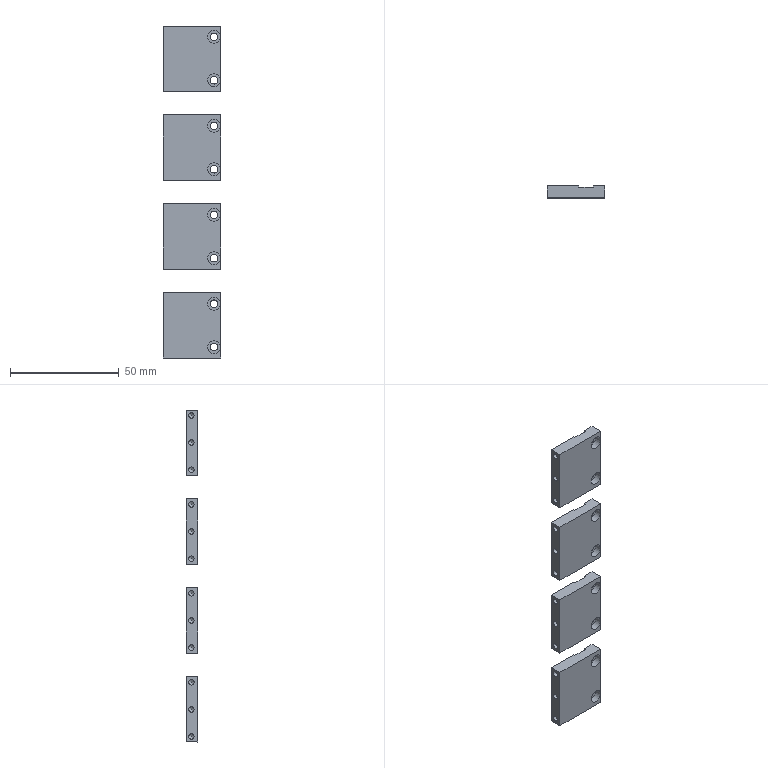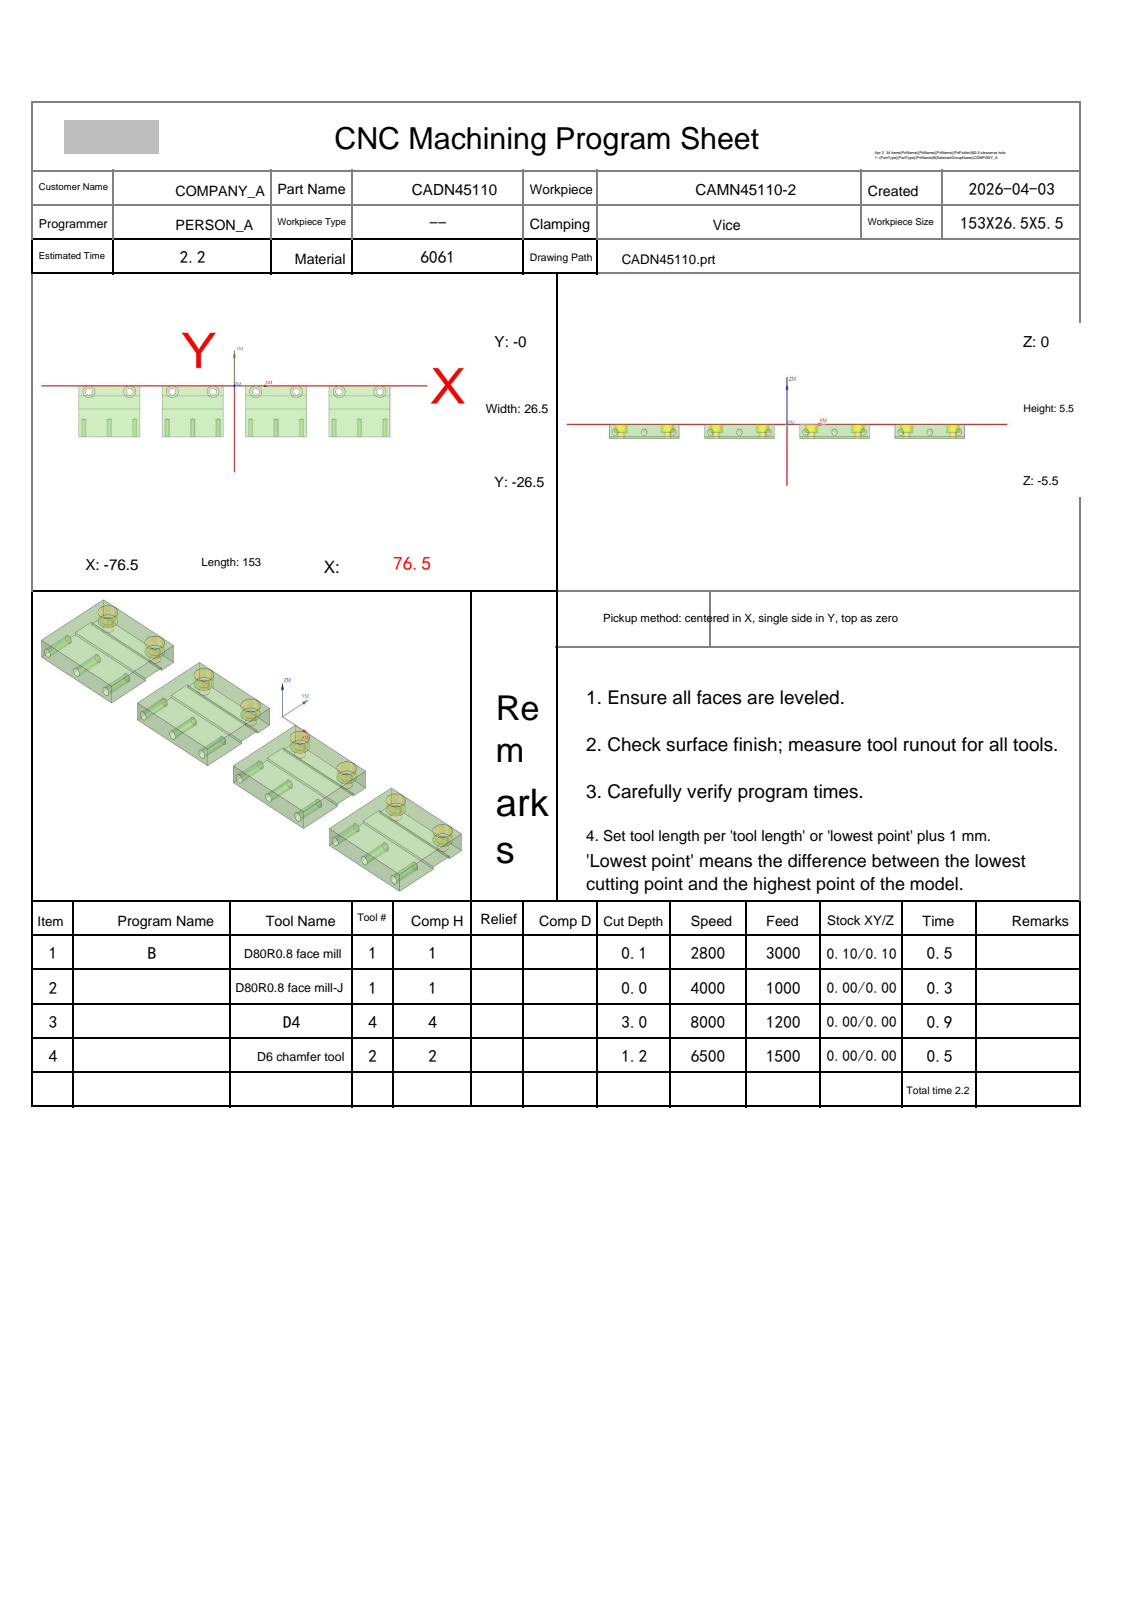NC program | NX | posted by the shop | part box 26.5 x 5.5 x 153 mm
Whole program:
%
O0001
(Machine time: 2.96 MIN)
(===Total Tool:3===)
(T1=D80R0.8 face mill D=80.  R=0.8  D-  H01 Z=-0.   )
(T4=D4      D=4.   R=0.   D-  H04 Z=-3.   )
(T2=D6 chamfer tool   D=6.   R=0.   D-  H02 Z=-1.2  )
G80 G90 G17 G49 G40
G91 G28 Z0
M01
N1 T01 M06
(D80R0.8 face mill  D=80. R=0.8 H=01 ce=0.10 di=0.10)
G00 G90 G54 X128.597 Y-13.25 M03 S2800
G43 H01 Z20.
M08
Z4.02
G01 Z2.02 F3000.
X116.597
X-116.597
X-128.597
Z4.02
G00 X128.597
Z3.54
G01 Z1.54
X116.597
X-116.597
X-128.597
Z3.54
G00 X128.597
Z3.06
G01 Z1.06
X116.597
X-116.597
X-128.597
Z3.06
G00 X128.597
Z2.58
G01 Z.58
X116.597
X-116.597
X-128.597
Z2.58
G00 Z20.
X128.597
Z2.1
G01 Z.1
X116.597
X-116.597
X-128.597
Z2.1
G00 Z20.
G91 G28 Z0.0
M05
M09
G91 G28 Z0.0
M01
N2 T01 M06
(D80R0.8 face mill-J  D=80. R=0.8 H=01 ce=0.00 di=0.00)
G00 G90 G54 X128.499 Y-13.25 M03 S4000
G43 H01 Z20.
M08
Z2.
G01 Z0.0 F1000.
X116.499
X-116.499
X-128.499
Z2.
G00 Z20.
G91 G28 Z0.0
M05
M09
G91 G28 Z0.0
M01
N3 T04 M06
(D4  D=4. R=0. H=04 ce=0.07 di=0.00)
G00 G90 G54 X-51.5 Y-3.1 M03 S8000
G43 H04 Z20.
M08
Z.3
G03 X-51.035 Y-2.635 I0.0 J.465 F1200.
X-51.5 Y-2.17 I-.465 J0.0
X-51.5 Y-2.17 Z.1 I0.0 J-.93
X-51.5 Y-2.17 Z-.1 I0.0 J-.93
X-51.5 Y-2.17 Z-.3 I0.0 J-.93
X-51.5 Y-2.17 Z-.5 I0.0 J-.93
X-51.5 Y-2.17 Z-.7 I0.0 J-.93
X-51.5 Y-2.17 Z-.9 I0.0 J-.93
X-51.5 Y-2.17 Z-1.1 I0.0 J-.93
X-51.5 Y-2.17 Z-1.3 I0.0 J-.93
X-51.5 Y-2.17 Z-1.5 I0.0 J-.93
X-51.5 Y-2.17 Z-1.7 I0.0 J-.93
X-51.5 Y-2.17 Z-1.9 I0.0 J-.93
X-51.5 Y-2.17 Z-2.1 I0.0 J-.93
X-51.5 Y-2.17 Z-2.3 I0.0 J-.93
X-51.5 Y-2.17 Z-2.5 I0.0 J-.93
X-51.5 Y-2.17 Z-2.7 I0.0 J-.93
X-51.5 Y-2.17 Z-2.9 I0.0 J-.93
X-51.5 Y-4.03 Z-3. I0.0 J-.93
X-50.57 Y-3.1 I0.0 J.93
X-51.5 Y-2.17 I-.93 J0.0
X-52.43 Y-3.1 I0.0 J-.93
X-51.5 Y-4.03 I.93 J0.0
X-51.035 Y-3.565 I0.0 J.465
X-51.5 Y-3.1 I-.465 J0.0
G00 Z20.
X-71.5
Z.3
G03 X-71.035 Y-2.635 I0.0 J.465
X-71.5 Y-2.17 I-.465 J0.0
X-71.5 Y-2.17 Z.1 I0.0 J-.93
X-71.5 Y-2.17 Z-.1 I0.0 J-.93
X-71.5 Y-2.17 Z-.3 I0.0 J-.93
X-71.5 Y-2.17 Z-.5 I0.0 J-.93
X-71.5 Y-2.17 Z-.7 I0.0 J-.93
X-71.5 Y-2.17 Z-.9 I0.0 J-.93
X-71.5 Y-2.17 Z-1.1 I0.0 J-.93
X-71.5 Y-2.17 Z-1.3 I0.0 J-.93
X-71.5 Y-2.17 Z-1.5 I0.0 J-.93
X-71.5 Y-2.17 Z-1.7 I0.0 J-.93
X-71.5 Y-2.17 Z-1.9 I0.0 J-.93
X-71.5 Y-2.17 Z-2.1 I0.0 J-.93
X-71.5 Y-2.17 Z-2.3 I0.0 J-.93
X-71.5 Y-2.17 Z-2.5 I0.0 J-.93
X-71.5 Y-2.17 Z-2.7 I0.0 J-.93
X-71.5 Y-2.17 Z-2.9 I0.0 J-.93
X-71.5 Y-4.03 Z-3. I0.0 J-.93
X-70.57 Y-3.1 I0.0 J.93
X-71.5 Y-2.17 I-.93 J0.0
X-72.43 Y-3.1 I0.0 J-.93
X-71.5 Y-4.03 I.93 J0.0
X-71.035 Y-3.565 I0.0 J.465
X-71.5 Y-3.1 I-.465 J0.0
G00 Z20.
X-30.5
Z.3
G03 X-30.035 Y-2.635 I0.0 J.465
X-30.5 Y-2.17 I-.465 J0.0
X-30.5 Y-2.17 Z.1 I0.0 J-.93
X-30.5 Y-2.17 Z-.1 I0.0 J-.93
X-30.5 Y-2.17 Z-.3 I0.0 J-.93
X-30.5 Y-2.17 Z-.5 I0.0 J-.93
X-30.5 Y-2.17 Z-.7 I0.0 J-.93
X-30.5 Y-2.17 Z-.9 I0.0 J-.93
X-30.5 Y-2.17 Z-1.1 I0.0 J-.93
X-30.5 Y-2.17 Z-1.3 I0.0 J-.93
X-30.5 Y-2.17 Z-1.5 I0.0 J-.93
X-30.5 Y-2.17 Z-1.7 I0.0 J-.93
X-30.5 Y-2.17 Z-1.9 I0.0 J-.93
X-30.5 Y-2.17 Z-2.1 I0.0 J-.93
X-30.5 Y-2.17 Z-2.3 I0.0 J-.93
X-30.5 Y-2.17 Z-2.5 I0.0 J-.93
X-30.5 Y-2.17 Z-2.7 I0.0 J-.93
X-30.5 Y-2.17 Z-2.9 I0.0 J-.93
X-30.5 Y-4.03 Z-3. I0.0 J-.93
X-29.57 Y-3.1 I0.0 J.93
X-30.5 Y-2.17 I-.93 J0.0
X-31.43 Y-3.1 I0.0 J-.93
X-30.5 Y-4.03 I.93 J0.0
X-30.035 Y-3.565 I0.0 J.465
X-30.5 Y-3.1 I-.465 J0.0
G00 Z20.
X-10.5
Z.3
G03 X-10.035 Y-2.635 I0.0 J.465
X-10.5 Y-2.17 I-.465 J0.0
X-10.5 Y-2.17 Z.1 I0.0 J-.93
X-10.5 Y-2.17 Z-.1 I0.0 J-.93
X-10.5 Y-2.17 Z-.3 I0.0 J-.93
X-10.5 Y-2.17 Z-.5 I0.0 J-.93
X-10.5 Y-2.17 Z-.7 I0.0 J-.93
X-10.5 Y-2.17 Z-.9 I0.0 J-.93
X-10.5 Y-2.17 Z-1.1 I0.0 J-.93
X-10.5 Y-2.17 Z-1.3 I0.0 J-.93
X-10.5 Y-2.17 Z-1.5 I0.0 J-.93
X-10.5 Y-2.17 Z-1.7 I0.0 J-.93
X-10.5 Y-2.17 Z-1.9 I0.0 J-.93
X-10.5 Y-2.17 Z-2.1 I0.0 J-.93
X-10.5 Y-2.17 Z-2.3 I0.0 J-.93
X-10.5 Y-2.17 Z-2.5 I0.0 J-.93
X-10.5 Y-2.17 Z-2.7 I0.0 J-.93
X-10.5 Y-2.17 Z-2.9 I0.0 J-.93
X-10.5 Y-4.03 Z-3. I0.0 J-.93
X-9.57 Y-3.1 I0.0 J.93
X-10.5 Y-2.17 I-.93 J0.0
X-11.43 Y-3.1 I0.0 J-.93
X-10.5 Y-4.03 I.93 J0.0
X-10.035 Y-3.565 I0.0 J.465
X-10.5 Y-3.1 I-.465 J0.0
G00 Z20.
X10.5
Z.3
G03 X10.965 Y-2.635 I0.0 J.465
X10.5 Y-2.17 I-.465 J0.0
X10.5 Y-2.17 Z.1 I0.0 J-.93
X10.5 Y-2.17 Z-.1 I0.0 J-.93
X10.5 Y-2.17 Z-.3 I0.0 J-.93
X10.5 Y-2.17 Z-.5 I0.0 J-.93
X10.5 Y-2.17 Z-.7 I0.0 J-.93
X10.5 Y-2.17 Z-.9 I0.0 J-.93
X10.5 Y-2.17 Z-1.1 I0.0 J-.93
X10.5 Y-2.17 Z-1.3 I0.0 J-.93
X10.5 Y-2.17 Z-1.5 I0.0 J-.93
X10.5 Y-2.17 Z-1.7 I0.0 J-.93
X10.5 Y-2.17 Z-1.9 I0.0 J-.93
X10.5 Y-2.17 Z-2.1 I0.0 J-.93
X10.5 Y-2.17 Z-2.3 I0.0 J-.93
X10.5 Y-2.17 Z-2.5 I0.0 J-.93
X10.5 Y-2.17 Z-2.7 I0.0 J-.93
X10.5 Y-2.17 Z-2.9 I0.0 J-.93
X10.5 Y-4.03 Z-3. I0.0 J-.93
X11.43 Y-3.1 I0.0 J.93
X10.5 Y-2.17 I-.93 J0.0
X9.57 Y-3.1 I0.0 J-.93
X10.5 Y-4.03 I.93 J0.0
X10.965 Y-3.565 I0.0 J.465
X10.5 Y-3.1 I-.465 J0.0
G00 Z20.
X30.5
Z.3
G03 X30.965 Y-2.635 I0.0 J.465
X30.5 Y-2.17 I-.465 J0.0
X30.5 Y-2.17 Z.1 I0.0 J-.93
X30.5 Y-2.17 Z-.1 I0.0 J-.93
X30.5 Y-2.17 Z-.3 I0.0 J-.93
X30.5 Y-2.17 Z-.5 I0.0 J-.93
X30.5 Y-2.17 Z-.7 I0.0 J-.93
X30.5 Y-2.17 Z-.9 I0.0 J-.93
X30.5 Y-2.17 Z-1.1 I0.0 J-.93
X30.5 Y-2.17 Z-1.3 I0.0 J-.93
X30.5 Y-2.17 Z-1.5 I0.0 J-.93
X30.5 Y-2.17 Z-1.7 I0.0 J-.93
X30.5 Y-2.17 Z-1.9 I0.0 J-.93
X30.5 Y-2.17 Z-2.1 I0.0 J-.93
X30.5 Y-2.17 Z-2.3 I0.0 J-.93
X30.5 Y-2.17 Z-2.5 I0.0 J-.93
X30.5 Y-2.17 Z-2.7 I0.0 J-.93
X30.5 Y-2.17 Z-2.9 I0.0 J-.93
X30.5 Y-4.03 Z-3. I0.0 J-.93
X31.43 Y-3.1 I0.0 J.93
X30.5 Y-2.17 I-.93 J0.0
X29.57 Y-3.1 I0.0 J-.93
X30.5 Y-4.03 I.93 J0.0
X30.965 Y-3.565 I0.0 J.465
X30.5 Y-3.1 I-.465 J0.0
G00 Z20.
X51.5
Z.3
G03 X51.965 Y-2.635 I0.0 J.465
X51.5 Y-2.17 I-.465 J0.0
X51.5 Y-2.17 Z.1 I0.0 J-.93
X51.5 Y-2.17 Z-.1 I0.0 J-.93
X51.5 Y-2.17 Z-.3 I0.0 J-.93
X51.5 Y-2.17 Z-.5 I0.0 J-.93
X51.5 Y-2.17 Z-.7 I0.0 J-.93
X51.5 Y-2.17 Z-.9 I0.0 J-.93
X51.5 Y-2.17 Z-1.1 I0.0 J-.93
X51.5 Y-2.17 Z-1.3 I0.0 J-.93
X51.5 Y-2.17 Z-1.5 I0.0 J-.93
X51.5 Y-2.17 Z-1.7 I0.0 J-.93
X51.5 Y-2.17 Z-1.9 I0.0 J-.93
X51.5 Y-2.17 Z-2.1 I0.0 J-.93
X51.5 Y-2.17 Z-2.3 I0.0 J-.93
X51.5 Y-2.17 Z-2.5 I0.0 J-.93
X51.5 Y-2.17 Z-2.7 I0.0 J-.93
X51.5 Y-2.17 Z-2.9 I0.0 J-.93
X51.5 Y-4.03 Z-3. I0.0 J-.93
X52.43 Y-3.1 I0.0 J.93
X51.5 Y-2.17 I-.93 J0.0
X50.57 Y-3.1 I0.0 J-.93
X51.5 Y-4.03 I.93 J0.0
X51.965 Y-3.565 I0.0 J.465
X51.5 Y-3.1 I-.465 J0.0
G00 Z20.
X71.5
Z.3
G03 X71.965 Y-2.635 I0.0 J.465
X71.5 Y-2.17 I-.465 J0.0
X71.5 Y-2.17 Z.1 I0.0 J-.93
X71.5 Y-2.17 Z-.1 I0.0 J-.93
X71.5 Y-2.17 Z-.3 I0.0 J-.93
X71.5 Y-2.17 Z-.5 I0.0 J-.93
X71.5 Y-2.17 Z-.7 I0.0 J-.93
X71.5 Y-2.17 Z-.9 I0.0 J-.93
X71.5 Y-2.17 Z-1.1 I0.0 J-.93
X71.5 Y-2.17 Z-1.3 I0.0 J-.93
X71.5 Y-2.17 Z-1.5 I0.0 J-.93
X71.5 Y-2.17 Z-1.7 I0.0 J-.93
X71.5 Y-2.17 Z-1.9 I0.0 J-.93
X71.5 Y-2.17 Z-2.1 I0.0 J-.93
X71.5 Y-2.17 Z-2.3 I0.0 J-.93
X71.5 Y-2.17 Z-2.5 I0.0 J-.93
X71.5 Y-2.17 Z-2.7 I0.0 J-.93
X71.5 Y-2.17 Z-2.9 I0.0 J-.93
X71.5 Y-4.03 Z-3. I0.0 J-.93
X72.43 Y-3.1 I0.0 J.93
X71.5 Y-2.17 I-.93 J0.0
X70.57 Y-3.1 I0.0 J-.93
X71.5 Y-4.03 I.93 J0.0
X71.965 Y-3.565 I0.0 J.465
X71.5 Y-3.1 I-.465 J0.0
G00 Z20.
G00 G90 X-51.5 Y-3.1 M03 S8000
Z20.
Z-3.
G01 X-51.228 Y-2.532 F600.
X-51.198 Y-2.402
G03 X-51.5 Y-2.1 I-.302 J0.0
X-52.5 Y-3.1 I0.0 J-1.
X-51.5 Y-4.1 I1. J0.0
X-50.5 Y-3.1 I0.0 J1.
X-51.5 Y-2.1 I-1. J0.0
X-51.979 Y-2.222 I0.0 J-1.
X-52.136 Y-2.487 I.145 J-.265
X-52.011 Y-2.732 I.302 J0.0
G01 X-51.5 Y-3.1
G00 Z20.
X-71.5
Z-3.
G01 X-71.228 Y-2.532
X-71.198 Y-2.402
G03 X-71.5 Y-2.1 I-.302 J0.0
X-72.5 Y-3.1 I0.0 J-1.
X-71.5 Y-4.1 I1. J0.0
X-70.5 Y-3.1 I0.0 J1.
X-71.5 Y-2.1 I-1. J0.0
X-71.979 Y-2.222 I0.0 J-1.
X-72.136 Y-2.487 I.145 J-.265
X-72.011 Y-2.732 I.302 J0.0
G01 X-71.5 Y-3.1
G00 Z20.
X-30.5
Z-3.
G01 X-30.228 Y-2.532
X-30.198 Y-2.402
G03 X-30.5 Y-2.1 I-.302 J0.0
X-31.5 Y-3.1 I0.0 J-1.
X-30.5 Y-4.1 I1. J0.0
X-29.5 Y-3.1 I0.0 J1.
X-30.5 Y-2.1 I-1. J0.0
X-30.979 Y-2.222 I0.0 J-1.
X-31.136 Y-2.487 I.145 J-.265
X-31.011 Y-2.732 I.302 J0.0
G01 X-30.5 Y-3.1
G00 Z20.
X-10.5
Z-3.
G01 X-10.228 Y-2.532
X-10.198 Y-2.402
G03 X-10.5 Y-2.1 I-.302 J0.0
X-11.5 Y-3.1 I0.0 J-1.
X-10.5 Y-4.1 I1. J0.0
X-9.5 Y-3.1 I0.0 J1.
X-10.5 Y-2.1 I-1. J0.0
X-10.979 Y-2.222 I0.0 J-1.
X-11.136 Y-2.487 I.145 J-.265
X-11.011 Y-2.732 I.302 J0.0
G01 X-10.5 Y-3.1
G00 Z20.
X10.5
Z-3.
G01 X10.772 Y-2.532
X10.802 Y-2.402
G03 X10.5 Y-2.1 I-.302 J0.0
X9.5 Y-3.1 I0.0 J-1.
X10.5 Y-4.1 I1. J0.0
X11.5 Y-3.1 I0.0 J1.
X10.5 Y-2.1 I-1. J0.0
X10.021 Y-2.222 I0.0 J-1.
X9.864 Y-2.487 I.145 J-.265
X9.989 Y-2.732 I.302 J0.0
G01 X10.5 Y-3.1
G00 Z20.
X30.5
Z-3.
G01 X30.772 Y-2.532
X30.802 Y-2.402
G03 X30.5 Y-2.1 I-.302 J0.0
X29.5 Y-3.1 I0.0 J-1.
X30.5 Y-4.1 I1. J0.0
X31.5 Y-3.1 I0.0 J1.
X30.5 Y-2.1 I-1. J0.0
X30.021 Y-2.222 I0.0 J-1.
X29.864 Y-2.487 I.145 J-.265
X29.989 Y-2.732 I.302 J0.0
G01 X30.5 Y-3.1
G00 Z20.
X51.5
Z-3.
G01 X51.772 Y-2.532
X51.802 Y-2.402
G03 X51.5 Y-2.1 I-.302 J0.0
X50.5 Y-3.1 I0.0 J-1.
X51.5 Y-4.1 I1. J0.0
X52.5 Y-3.1 I0.0 J1.
X51.5 Y-2.1 I-1. J0.0
X51.021 Y-2.222 I0.0 J-1.
X50.864 Y-2.487 I.145 J-.265
X50.989 Y-2.732 I.302 J0.0
G01 X51.5 Y-3.1
G00 Z20.
X71.5
Z-3.
G01 X71.772 Y-2.532
X71.802 Y-2.402
G03 X71.5 Y-2.1 I-.302 J0.0
X70.5 Y-3.1 I0.0 J-1.
X71.5 Y-4.1 I1. J0.0
X72.5 Y-3.1 I0.0 J1.
X71.5 Y-2.1 I-1. J0.0
X71.021 Y-2.222 I0.0 J-1.
X70.864 Y-2.487 I.145 J-.265
X70.989 Y-2.732 I.302 J0.0
G01 X71.5 Y-3.1
G00 Z20.
G91 G28 Z0.0
M05
M09
G91 G28 Z0.0
M01
N4 T02 M06
(D6 chamfer tool  D=6. R=0. H=02 ce=0.00 di=0.00)
G00 G90 G54 X61.886 Y-27.727 M03 S6500
G43 H02 Z20.
M08
Z.172
G01 Z-1.2 F1500.
G03 X61.6 Y-27.527 I-1.286 J-1.532
G01 X61.554 Y-27.497
X61.5 Y-27.5
X46.5
G02 X45.5 Y-26.5 I0.0 J1.
G01 Y0.0
G02 X46.5 Y1. I1. J0.0
G01 X76.5
G02 X77.5 Y0.0 I0.0 J-1.
G01 Y-26.5
G02 X76.5 Y-27.5 I-1. J0.0
G01 X61.5
X61.446 Y-27.497
X61.4 Y-27.527
G03 X61.114 Y-27.727 I1. J-1.732
G01 Z.172
G00 Z10.
X49.692 Y-2.696
Z.26
G01 Z-1.2
G03 X49.518 Y-2.998 I1.638 J-1.147
G01 X49.492 Y-3.046
X49.5 Y-3.1
G03 X51.5 Y-5.1 I2. J0.0
X53.5 Y-3.1 I0.0 J2.
X51.5 Y-1.1 I-2. J0.0
X49.53 Y-2.753 I0.0 J-2.
G01 X49.5 Y-3.1
X49.492 Y-3.154
X49.518 Y-3.202
G03 X49.692 Y-3.504 I1.813 J.845
G01 Z.257
G00 Z10.
X69.692 Y-2.696
Z.26
G01 Z-1.2
G03 X69.518 Y-2.998 I1.638 J-1.147
G01 X69.492 Y-3.046
X69.5 Y-3.1
G03 X71.5 Y-5.1 I2. J0.0
X73.5 Y-3.1 I0.0 J2.
X71.5 Y-1.1 I-2. J0.0
X69.53 Y-2.753 I0.0 J-2.
G01 X69.5 Y-3.1
X69.492 Y-3.154
X69.518 Y-3.202
G03 X69.692 Y-3.504 I1.813 J.845
G01 Z.257
G00 Z10.
X20.114 Y1.227
Z.172
G01 Z-1.2
G03 X20.4 Y1.027 I1.286 J1.532
G01 X20.446 Y.997
X20.5 Y1.
X35.5
G02 X36.5 Y0.0 I0.0 J-1.
G01 Y-26.5
G02 X35.5 Y-27.5 I-1. J0.0
G01 X5.5
G02 X4.5 Y-26.5 I0.0 J1.
G01 Y0.0
G02 X5.5 Y1. I1. J0.0
G01 X20.5
X20.554 Y.997
X20.6 Y1.027
G03 X20.886 Y1.227 I-1. J1.732
G01 Z.172
G00 Z10.
X8.692 Y-2.696
Z.26
G01 Z-1.2
G03 X8.518 Y-2.998 I1.638 J-1.147
G01 X8.492 Y-3.046
X8.5 Y-3.1
G03 X10.5 Y-5.1 I2. J0.0
X12.5 Y-3.1 I0.0 J2.
X10.5 Y-1.1 I-2. J0.0
X8.53 Y-2.753 I0.0 J-2.
G01 X8.5 Y-3.1
X8.492 Y-3.154
X8.518 Y-3.202
G03 X8.692 Y-3.504 I1.813 J.845
G01 Z.257
G00 Z10.
X28.692 Y-2.696
Z.26
G01 Z-1.2
G03 X28.518 Y-2.998 I1.638 J-1.147
G01 X28.492 Y-3.046
X28.5 Y-3.1
G03 X30.5 Y-5.1 I2. J0.0
X32.5 Y-3.1 I0.0 J2.
X30.5 Y-1.1 I-2. J0.0
X28.53 Y-2.753 I0.0 J-2.
G01 X28.5 Y-3.1
X28.492 Y-3.154
X28.518 Y-3.202
G03 X28.692 Y-3.504 I1.813 J.845
G01 Z.257
G00 Z10.
X-20.886 Y1.227
Z.172
G01 Z-1.2
G03 X-20.6 Y1.027 I1.286 J1.532
G01 X-20.554 Y.997
X-20.5 Y1.
X-5.5
G02 X-4.5 Y0.0 I0.0 J-1.
G01 Y-26.5
G02 X-5.5 Y-27.5 I-1. J0.0
G01 X-35.5
G02 X-36.5 Y-26.5 I0.0 J1.
G01 Y0.0
G02 X-35.5 Y1. I1. J0.0
G01 X-20.5
X-20.446 Y.997
X-20.4 Y1.027
G03 X-20.114 Y1.227 I-1. J1.732
G01 Z.172
G00 Z10.
X-32.308 Y-2.696
Z.26
G01 Z-1.2
G03 X-32.482 Y-2.998 I1.638 J-1.147
G01 X-32.508 Y-3.046
X-32.5 Y-3.1
G03 X-30.5 Y-5.1 I2. J0.0
X-28.5 Y-3.1 I0.0 J2.
X-30.5 Y-1.1 I-2. J0.0
X-32.47 Y-2.753 I0.0 J-2.
G01 X-32.5 Y-3.1
X-32.508 Y-3.154
X-32.482 Y-3.202
G03 X-32.308 Y-3.504 I1.813 J.845
G01 Z.257
G00 Z10.
X-12.308 Y-2.696
Z.26
G01 Z-1.2
G03 X-12.482 Y-2.998 I1.638 J-1.147
G01 X-12.508 Y-3.046
X-12.5 Y-3.1
G03 X-10.5 Y-5.1 I2. J0.0
X-8.5 Y-3.1 I0.0 J2.
X-10.5 Y-1.1 I-2. J0.0
X-12.47 Y-2.753 I0.0 J-2.
G01 X-12.5 Y-3.1
X-12.508 Y-3.154
X-12.482 Y-3.202
G03 X-12.308 Y-3.504 I1.813 J.845
G01 Z.257
G00 Z10.
X-61.886 Y1.227
Z.172
G01 Z-1.2
G03 X-61.6 Y1.027 I1.286 J1.532
G01 X-61.554 Y.997
X-61.5 Y1.
X-46.5
G02 X-45.5 Y0.0 I0.0 J-1.
G01 Y-26.5
G02 X-46.5 Y-27.5 I-1. J0.0
G01 X-76.5
G02 X-77.5 Y-26.5 I0.0 J1.
G01 Y0.0
G02 X-76.5 Y1. I1. J0.0
G01 X-61.5
X-61.446 Y.997
X-61.4 Y1.027
G03 X-61.114 Y1.227 I-1. J1.732
G01 Z.172
G00 Z10.
X-73.308 Y-2.696
Z.26
G01 Z-1.2
G03 X-73.482 Y-2.998 I1.638 J-1.147
G01 X-73.508 Y-3.046
X-73.5 Y-3.1
G03 X-71.5 Y-5.1 I2. J0.0
X-69.5 Y-3.1 I0.0 J2.
X-71.5 Y-1.1 I-2. J0.0
X-73.47 Y-2.753 I0.0 J-2.
G01 X-73.5 Y-3.1
X-73.508 Y-3.154
X-73.482 Y-3.202
G03 X-73.308 Y-3.504 I1.813 J.845
G01 Z.257
G00 Z10.
X-53.308 Y-2.696
Z.26
G01 Z-1.2
G03 X-53.482 Y-2.998 I1.638 J-1.147
G01 X-53.508 Y-3.046
X-53.5 Y-3.1
G03 X-51.5 Y-5.1 I2. J0.0
X-49.5 Y-3.1 I0.0 J2.
X-51.5 Y-1.1 I-2. J0.0
X-53.47 Y-2.753 I0.0 J-2.
G01 X-53.5 Y-3.1
X-53.508 Y-3.154
X-53.482 Y-3.202
G03 X-53.308 Y-3.504 I1.813 J.845
G01 Z.257
G00 Z20.
M05
M09
G91 G28 Z0.0
G91 G28 Y0.0
M30
%